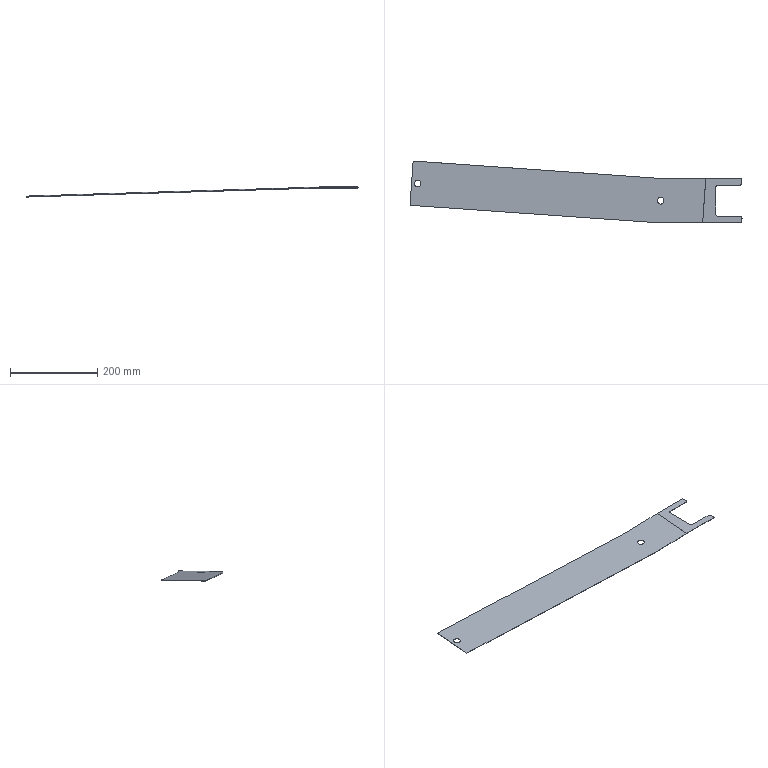Part | SolidWorks | features BaseBody 1 | 1 solid | 28 faces | box 762.872 x 142.38 x 23.327 mm | volume 58351 mm3 | plane 16 | cylinder 10 | spline 2 | commonest cylinder face diameters 10 x4 15.3 x4 2 x1 3.6 x1
STEP:
#1=CARTESIAN_POINT('',(1.188,13.037,-3.513));
#2=VERTEX_POINT('',#1);
#3=CARTESIAN_POINT('',(-14.105,13.037,-3.999));
#4=VERTEX_POINT('',#3);
#5=CARTESIAN_POINT('',(-6.458,13.037,-3.756));
#6=DIRECTION('',(0.03175,0.01522,-0.9994));
#7=DIRECTION('',(0.9995,0.,0.03176));
#8=AXIS2_PLACEMENT_3D('',#5,#6,#7);
#9=CIRCLE('',#8,7.65);
#10=EDGE_CURVE('',#2,#4,#9,.T.);
#11=ORIENTED_EDGE('',*,*,#10,.T.);
#12=CARTESIAN_POINT('',(-14.13,13.025,-3.199));
#13=VERTEX_POINT('',#12);
#14=CARTESIAN_POINT('',(-14.105,13.037,-3.999));
#15=DIRECTION('',(-0.03175,-0.01522,0.9994));
#16=VECTOR('',#15,1000.);
#17=LINE('',#14,#16);
#18=EDGE_CURVE('',#4,#13,#17,.T.);
#19=ORIENTED_EDGE('',*,*,#18,.T.);
#20=CARTESIAN_POINT('',(1.162,13.025,-2.713));
#21=VERTEX_POINT('',#20);
#22=CARTESIAN_POINT('',(-6.484,13.025,-2.956));
#23=DIRECTION('',(-0.03175,-0.01522,0.9994));
#24=DIRECTION('',(0.9995,0.,0.03176));
#25=AXIS2_PLACEMENT_3D('',#22,#23,#24);
#26=CIRCLE('',#25,7.65);
#27=EDGE_CURVE('',#13,#21,#26,.T.);
#28=ORIENTED_EDGE('',*,*,#27,.T.);
#29=CARTESIAN_POINT('',(1.188,13.037,-3.513));
#30=DIRECTION('',(-0.03175,-0.01522,0.9994));
#31=VECTOR('',#30,1000.);
#32=LINE('',#29,#31);
#33=EDGE_CURVE('',#2,#21,#32,.T.);
#34=ORIENTED_EDGE('',*,*,#33,.F.);
#35=EDGE_LOOP('',(#11,#19,#28,#34));
#36=FACE_OUTER_BOUND('',#35,.T.);
#37=CARTESIAN_POINT('',(-6.458,13.037,-3.756));
#38=DIRECTION('',(-0.03175,-0.01522,0.9994));
#39=DIRECTION('',(0.9995,0.,0.03176));
#40=AXIS2_PLACEMENT_3D('',#37,#38,#39);
#41=CYLINDRICAL_SURFACE('',#40,7.65);
#42=ADVANCED_FACE('',(#36),#41,.F.);
#43=CARTESIAN_POINT('',(-557.165,52.386,-20.653));
#44=VERTEX_POINT('',#43);
#45=CARTESIAN_POINT('',(-572.457,52.386,-21.139));
#46=VERTEX_POINT('',#45);
#47=CARTESIAN_POINT('',(-564.811,52.386,-20.896));
#48=DIRECTION('',(0.03175,0.01522,-0.9994));
#49=DIRECTION('',(0.9995,0.,0.03176));
#50=AXIS2_PLACEMENT_3D('',#47,#48,#49);
#51=CIRCLE('',#50,7.65);
#52=EDGE_CURVE('',#44,#46,#51,.T.);
#53=ORIENTED_EDGE('',*,*,#52,.T.);
#54=CARTESIAN_POINT('',(-572.483,52.374,-20.34));
#55=VERTEX_POINT('',#54);
#56=CARTESIAN_POINT('',(-572.457,52.386,-21.139));
#57=DIRECTION('',(-0.03175,-0.01522,0.9994));
#58=VECTOR('',#57,1000.);
#59=LINE('',#56,#58);
#60=EDGE_CURVE('',#46,#55,#59,.T.);
#61=ORIENTED_EDGE('',*,*,#60,.T.);
#62=CARTESIAN_POINT('',(-557.191,52.374,-19.854));
#63=VERTEX_POINT('',#62);
#64=CARTESIAN_POINT('',(-564.837,52.374,-20.097));
#65=DIRECTION('',(0.03175,0.01522,-0.9994));
#66=DIRECTION('',(0.9995,0.,0.03176));
#67=AXIS2_PLACEMENT_3D('',#64,#65,#66);
#68=CIRCLE('',#67,7.65);
#69=EDGE_CURVE('',#63,#55,#68,.T.);
#70=ORIENTED_EDGE('',*,*,#69,.F.);
#71=CARTESIAN_POINT('',(-557.165,52.386,-20.653));
#72=DIRECTION('',(-0.03175,-0.01522,0.9994));
#73=VECTOR('',#72,1000.);
#74=LINE('',#71,#73);
#75=EDGE_CURVE('',#44,#63,#74,.T.);
#76=ORIENTED_EDGE('',*,*,#75,.F.);
#77=EDGE_LOOP('',(#53,#61,#70,#76));
#78=FACE_OUTER_BOUND('',#77,.T.);
#79=CARTESIAN_POINT('',(-564.811,52.386,-20.896));
#80=DIRECTION('',(-0.03175,-0.01522,0.9994));
#81=DIRECTION('',(0.9995,0.,0.03176));
#82=AXIS2_PLACEMENT_3D('',#79,#80,#81);
#83=CYLINDRICAL_SURFACE('',#82,7.65);
#84=ADVANCED_FACE('',(#78),#83,.F.);
#85=ORIENTED_EDGE('',*,*,#18,.F.);
#86=CARTESIAN_POINT('',(-6.458,13.037,-3.756));
#87=DIRECTION('',(0.03175,0.01522,-0.9994));
#88=DIRECTION('',(0.9995,0.,0.03176));
#89=AXIS2_PLACEMENT_3D('',#86,#87,#88);
#90=CIRCLE('',#89,7.65);
#91=EDGE_CURVE('',#4,#2,#90,.T.);
#92=ORIENTED_EDGE('',*,*,#91,.T.);
#93=ORIENTED_EDGE('',*,*,#33,.T.);
#94=CARTESIAN_POINT('',(-6.484,13.025,-2.956));
#95=DIRECTION('',(-0.03175,-0.01522,0.9994));
#96=DIRECTION('',(0.9995,0.,0.03176));
#97=AXIS2_PLACEMENT_3D('',#94,#95,#96);
#98=CIRCLE('',#97,7.65);
#99=EDGE_CURVE('',#21,#13,#98,.T.);
#100=ORIENTED_EDGE('',*,*,#99,.T.);
#101=EDGE_LOOP('',(#85,#92,#93,#100));
#102=FACE_OUTER_BOUND('',#101,.T.);
#103=CARTESIAN_POINT('',(-6.458,13.037,-3.756));
#104=DIRECTION('',(-0.03175,-0.01522,0.9994));
#105=DIRECTION('',(0.9995,0.,0.03176));
#106=AXIS2_PLACEMENT_3D('',#103,#104,#105);
#107=CYLINDRICAL_SURFACE('',#106,7.65);
#108=ADVANCED_FACE('',(#102),#107,.F.);
#109=ORIENTED_EDGE('',*,*,#69,.T.);
#110=CARTESIAN_POINT('',(-564.837,52.374,-20.097));
#111=DIRECTION('',(0.03175,0.01522,-0.9994));
#112=DIRECTION('',(0.9995,0.,0.03176));
#113=AXIS2_PLACEMENT_3D('',#110,#111,#112);
#114=CIRCLE('',#113,7.65);
#115=EDGE_CURVE('',#55,#63,#114,.T.);
#116=ORIENTED_EDGE('',*,*,#115,.T.);
#117=EDGE_LOOP('',(#109,#116));
#118=FACE_BOUND('',#117,.T.);
#119=ORIENTED_EDGE('',*,*,#99,.F.);
#120=ORIENTED_EDGE('',*,*,#27,.F.);
#121=EDGE_LOOP('',(#119,#120));
#122=FACE_BOUND('',#121,.T.);
#123=CARTESIAN_POINT('',(-582.353,2.49,-21.413));
#124=VERTEX_POINT('',#123);
#125=CARTESIAN_POINT('',(-6.526,-38.091,-3.736));
#126=VERTEX_POINT('',#125);
#127=CARTESIAN_POINT('',(-582.353,2.49,-21.413));
#128=DIRECTION('',(0.9971,-0.07027,0.03061));
#129=VECTOR('',#128,1000.);
#130=LINE('',#127,#129);
#131=EDGE_CURVE('',#124,#126,#130,.T.);
#132=ORIENTED_EDGE('',*,*,#131,.T.);
#133=CARTESIAN_POINT('',(90.113,-38.141,-0.6667));
#134=VERTEX_POINT('',#133);
#135=CARTESIAN_POINT('',(-242.556,-37.968,-11.233));
#136=DIRECTION('',(0.9995,-0.0005189,0.03175));
#137=VECTOR('',#136,1000.);
#138=LINE('',#135,#137);
#139=EDGE_CURVE('',#126,#134,#138,.T.);
#140=ORIENTED_EDGE('',*,*,#139,.T.);
#141=CARTESIAN_POINT('',(97.245,63.844,1.113));
#142=VERTEX_POINT('',#141);
#143=CARTESIAN_POINT('',(90.113,-38.141,-0.6667));
#144=DIRECTION('',(0.06976,0.9974,0.01741));
#145=VECTOR('',#144,1000.);
#146=LINE('',#143,#145);
#147=EDGE_CURVE('',#134,#142,#146,.T.);
#148=ORIENTED_EDGE('',*,*,#147,.T.);
#149=CARTESIAN_POINT('',(-2.962,63.896,-2.069));
#150=VERTEX_POINT('',#149);
#151=CARTESIAN_POINT('',(-242.553,64.02,-9.68));
#152=DIRECTION('',(-0.9995,0.0005189,-0.03175));
#153=VECTOR('',#152,1000.);
#154=LINE('',#151,#153);
#155=EDGE_CURVE('',#142,#150,#154,.T.);
#156=ORIENTED_EDGE('',*,*,#155,.T.);
#157=CARTESIAN_POINT('',(-575.238,104.226,-19.637));
#158=VERTEX_POINT('',#157);
#159=CARTESIAN_POINT('',(-2.962,63.896,-2.069));
#160=DIRECTION('',(-0.9971,0.07027,-0.03061));
#161=VECTOR('',#160,1000.);
#162=LINE('',#159,#161);
#163=EDGE_CURVE('',#150,#158,#162,.T.);
#164=ORIENTED_EDGE('',*,*,#163,.T.);
#165=CARTESIAN_POINT('',(-575.238,104.226,-19.637));
#166=DIRECTION('',(-0.06976,-0.9974,-0.01741));
#167=VECTOR('',#166,1000.);
#168=LINE('',#165,#167);
#169=EDGE_CURVE('',#158,#124,#168,.T.);
#170=ORIENTED_EDGE('',*,*,#169,.T.);
#171=EDGE_LOOP('',(#132,#140,#148,#156,#164,#170));
#172=FACE_OUTER_BOUND('',#171,.T.);
#173=CARTESIAN_POINT('',(-586.427,105.084,-19.98));
#174=DIRECTION('',(-0.03175,-0.01522,0.9994));
#175=DIRECTION('',(-0.00003526,-0.9999,-0.01523));
#176=AXIS2_PLACEMENT_3D('',#173,#174,#175);
#177=PLANE('',#176);
#178=ADVANCED_FACE('',(#118,#122,#172),#177,.T.);
#179=ORIENTED_EDGE('',*,*,#52,.F.);
#180=CARTESIAN_POINT('',(-564.811,52.386,-20.896));
#181=DIRECTION('',(0.03175,0.01522,-0.9994));
#182=DIRECTION('',(0.9995,0.,0.03176));
#183=AXIS2_PLACEMENT_3D('',#180,#181,#182);
#184=CIRCLE('',#183,7.65);
#185=EDGE_CURVE('',#46,#44,#184,.T.);
#186=ORIENTED_EDGE('',*,*,#185,.F.);
#187=EDGE_LOOP('',(#179,#186));
#188=FACE_BOUND('',#187,.T.);
#189=ORIENTED_EDGE('',*,*,#10,.F.);
#190=ORIENTED_EDGE('',*,*,#91,.F.);
#191=EDGE_LOOP('',(#189,#190));
#192=FACE_BOUND('',#191,.T.);
#193=CARTESIAN_POINT('',(90.138,-38.129,-1.466));
#194=VERTEX_POINT('',#193);
#195=CARTESIAN_POINT('',(97.271,63.856,0.314));
#196=VERTEX_POINT('',#195);
#197=CARTESIAN_POINT('',(90.095,-38.741,-1.477));
#198=DIRECTION('',(0.06976,0.9974,0.01741));
#199=VECTOR('',#198,1000.);
#200=LINE('',#197,#199);
#201=EDGE_CURVE('',#194,#196,#200,.T.);
#202=ORIENTED_EDGE('',*,*,#201,.F.);
#203=CARTESIAN_POINT('',(-6.5,-38.079,-4.536));
#204=VERTEX_POINT('',#203);
#205=CARTESIAN_POINT('',(-242.531,-37.956,-12.033));
#206=DIRECTION('',(0.9995,-0.0005189,0.03175));
#207=VECTOR('',#206,1000.);
#208=LINE('',#205,#207);
#209=EDGE_CURVE('',#204,#194,#208,.T.);
#210=ORIENTED_EDGE('',*,*,#209,.F.);
#211=CARTESIAN_POINT('',(-582.328,2.502,-22.213));
#212=VERTEX_POINT('',#211);
#213=CARTESIAN_POINT('',(-582.328,2.502,-22.213));
#214=DIRECTION('',(0.9971,-0.07027,0.03061));
#215=VECTOR('',#214,1000.);
#216=LINE('',#213,#215);
#217=EDGE_CURVE('',#212,#204,#216,.T.);
#218=ORIENTED_EDGE('',*,*,#217,.F.);
#219=CARTESIAN_POINT('',(-575.213,104.238,-20.437));
#220=VERTEX_POINT('',#219);
#221=CARTESIAN_POINT('',(-575.213,104.238,-20.437));
#222=DIRECTION('',(-0.06976,-0.9974,-0.01741));
#223=VECTOR('',#222,1000.);
#224=LINE('',#221,#223);
#225=EDGE_CURVE('',#220,#212,#224,.T.);
#226=ORIENTED_EDGE('',*,*,#225,.F.);
#227=CARTESIAN_POINT('',(-2.937,63.908,-2.869));
#228=VERTEX_POINT('',#227);
#229=CARTESIAN_POINT('',(-2.937,63.908,-2.869));
#230=DIRECTION('',(-0.9971,0.07027,-0.03061));
#231=VECTOR('',#230,1000.);
#232=LINE('',#229,#231);
#233=EDGE_CURVE('',#228,#220,#232,.T.);
#234=ORIENTED_EDGE('',*,*,#233,.F.);
#235=CARTESIAN_POINT('',(-242.527,64.032,-10.479));
#236=DIRECTION('',(-0.9995,0.0005189,-0.03175));
#237=VECTOR('',#236,1000.);
#238=LINE('',#235,#237);
#239=EDGE_CURVE('',#196,#228,#238,.T.);
#240=ORIENTED_EDGE('',*,*,#239,.F.);
#241=EDGE_LOOP('',(#202,#210,#218,#226,#234,#240));
#242=FACE_OUTER_BOUND('',#241,.T.);
#243=CARTESIAN_POINT('',(-586.402,105.096,-20.779));
#244=DIRECTION('',(-0.03175,-0.01522,0.9994));
#245=DIRECTION('',(-0.00003526,-0.9999,-0.01523));
#246=AXIS2_PLACEMENT_3D('',#243,#244,#245);
#247=PLANE('',#246);
#248=ADVANCED_FACE('',(#188,#192,#242),#247,.F.);
#249=ORIENTED_EDGE('',*,*,#60,.F.);
#250=ORIENTED_EDGE('',*,*,#185,.T.);
#251=ORIENTED_EDGE('',*,*,#75,.T.);
#252=ORIENTED_EDGE('',*,*,#115,.F.);
#253=EDGE_LOOP('',(#249,#250,#251,#252));
#254=FACE_OUTER_BOUND('',#253,.T.);
#255=CARTESIAN_POINT('',(-564.811,52.386,-20.896));
#256=DIRECTION('',(-0.03175,-0.01522,0.9994));
#257=DIRECTION('',(0.9995,0.,0.03176));
#258=AXIS2_PLACEMENT_3D('',#255,#256,#257);
#259=CYLINDRICAL_SURFACE('',#258,7.65);
#260=ADVANCED_FACE('',(#254),#259,.F.);
#261=CARTESIAN_POINT('',(90.125,-38.135,-1.066));
#262=DIRECTION('',(0.03175,0.01522,-0.9994));
#263=VECTOR('',#262,1000.);
#264=LINE('',#261,#263);
#265=EDGE_CURVE('',#134,#194,#264,.T.);
#266=ORIENTED_EDGE('',*,*,#265,.F.);
#267=ORIENTED_EDGE('',*,*,#139,.F.);
#268=CARTESIAN_POINT('',(-6.513,-38.085,-4.136));
#269=DIRECTION('',(-0.03175,-0.01522,0.9994));
#270=VECTOR('',#269,1000.);
#271=LINE('',#268,#270);
#272=EDGE_CURVE('',#204,#126,#271,.T.);
#273=ORIENTED_EDGE('',*,*,#272,.F.);
#274=ORIENTED_EDGE('',*,*,#209,.T.);
#275=EDGE_LOOP('',(#266,#267,#273,#274));
#276=FACE_OUTER_BOUND('',#275,.T.);
#277=CARTESIAN_POINT('',(-6.5,-38.079,-4.536));
#278=DIRECTION('',(0.00003526,0.9999,0.01523));
#279=DIRECTION('',(-0.03175,-0.01522,0.9994));
#280=AXIS2_PLACEMENT_3D('',#277,#278,#279);
#281=PLANE('',#280);
#282=ADVANCED_FACE('',(#276),#281,.F.);
#283=CARTESIAN_POINT('',(-582.328,2.502,-22.213));
#284=DIRECTION('',(-0.03175,-0.01522,0.9994));
#285=VECTOR('',#284,1000.);
#286=LINE('',#283,#285);
#287=EDGE_CURVE('',#212,#124,#286,.T.);
#288=ORIENTED_EDGE('',*,*,#287,.F.);
#289=ORIENTED_EDGE('',*,*,#217,.T.);
#290=ORIENTED_EDGE('',*,*,#272,.T.);
#291=ORIENTED_EDGE('',*,*,#131,.F.);
#292=EDGE_LOOP('',(#288,#289,#290,#291));
#293=FACE_OUTER_BOUND('',#292,.T.);
#294=CARTESIAN_POINT('',(-3.044,-38.322,-4.434));
#295=DIRECTION('',(0.06976,0.9974,0.01741));
#296=DIRECTION('',(-0.997,0.07028,-0.03182));
#297=AXIS2_PLACEMENT_3D('',#294,#295,#296);
#298=PLANE('',#297);
#299=ADVANCED_FACE('',(#293),#298,.F.);
#300=CARTESIAN_POINT('',(-575.213,104.238,-20.437));
#301=DIRECTION('',(-0.03175,-0.01522,0.9994));
#302=VECTOR('',#301,1000.);
#303=LINE('',#300,#302);
#304=EDGE_CURVE('',#220,#158,#303,.T.);
#305=ORIENTED_EDGE('',*,*,#304,.F.);
#306=ORIENTED_EDGE('',*,*,#225,.T.);
#307=ORIENTED_EDGE('',*,*,#287,.T.);
#308=ORIENTED_EDGE('',*,*,#169,.F.);
#309=EDGE_LOOP('',(#305,#306,#307,#308));
#310=FACE_OUTER_BOUND('',#309,.T.);
#311=CARTESIAN_POINT('',(-582.371,1.878,-22.228));
#312=DIRECTION('',(0.9971,-0.07027,0.03061));
#313=DIRECTION('',(0.0703,0.9975,0.000008145));
#314=AXIS2_PLACEMENT_3D('',#311,#312,#313);
#315=PLANE('',#314);
#316=ADVANCED_FACE('',(#310),#315,.F.);
#317=CARTESIAN_POINT('',(-2.962,63.896,-2.069));
#318=DIRECTION('',(-0.03175,-0.01522,0.9994));
#319=VECTOR('',#318,1000.);
#320=LINE('',#317,#319);
#321=EDGE_CURVE('',#228,#150,#320,.T.);
#322=ORIENTED_EDGE('',*,*,#321,.F.);
#323=ORIENTED_EDGE('',*,*,#233,.T.);
#324=ORIENTED_EDGE('',*,*,#304,.T.);
#325=ORIENTED_EDGE('',*,*,#163,.F.);
#326=EDGE_LOOP('',(#322,#323,#324,#325));
#327=FACE_OUTER_BOUND('',#326,.T.);
#328=CARTESIAN_POINT('',(-578.623,104.491,-21.254));
#329=DIRECTION('',(-0.06976,-0.9974,-0.01741));
#330=DIRECTION('',(0.997,-0.07028,0.03182));
#331=AXIS2_PLACEMENT_3D('',#328,#329,#330);
#332=PLANE('',#331);
#333=ADVANCED_FACE('',(#327),#332,.F.);
#334=CARTESIAN_POINT('',(97.258,63.85,0.7137));
#335=DIRECTION('',(-0.03175,-0.01522,0.9994));
#336=VECTOR('',#335,1000.);
#337=LINE('',#334,#336);
#338=EDGE_CURVE('',#196,#142,#337,.T.);
#339=ORIENTED_EDGE('',*,*,#338,.F.);
#340=ORIENTED_EDGE('',*,*,#239,.T.);
#341=ORIENTED_EDGE('',*,*,#321,.T.);
#342=ORIENTED_EDGE('',*,*,#155,.F.);
#343=EDGE_LOOP('',(#339,#340,#341,#342));
#344=FACE_OUTER_BOUND('',#343,.T.);
#345=CARTESIAN_POINT('',(-2.962,63.896,-2.069));
#346=DIRECTION('',(-0.00003526,-0.9999,-0.01523));
#347=DIRECTION('',(0.03175,0.01522,-0.9994));
#348=AXIS2_PLACEMENT_3D('',#345,#346,#347);
#349=PLANE('',#348);
#350=ADVANCED_FACE('',(#344),#349,.F.);
#351=CARTESIAN_POINT('',(97.303,63.843,1.114));
#352=VERTEX_POINT('',#351);
#353=CARTESIAN_POINT('',(90.17,-38.142,-0.6658));
#354=VERTEX_POINT('',#353);
#355=CARTESIAN_POINT('',(93.736,12.849,0.2243));
#356=DIRECTION('',(-0.06976,-0.9974,-0.01741));
#357=VECTOR('',#356,1000.);
#358=LINE('',#355,#357);
#359=EDGE_CURVE('',#352,#354,#358,.T.);
#360=ORIENTED_EDGE('',*,*,#359,.F.);
#361=CARTESIAN_POINT('',(97.245,63.844,1.113));
#362=CARTESIAN_POINT('',(97.264,63.843,1.114));
#363=CARTESIAN_POINT('',(97.283,63.843,1.114));
#364=CARTESIAN_POINT('',(97.303,63.843,1.114));
#365=B_SPLINE_CURVE_WITH_KNOTS('',3,(#361,#362,#363,#364),.UNSPECIFIED.,.F.,.F.,(4,4),(0.,1.),.UNSPECIFIED.);
#366=EDGE_CURVE('',#142,#352,#365,.T.);
#367=ORIENTED_EDGE('',*,*,#366,.F.);
#368=ORIENTED_EDGE('',*,*,#147,.F.);
#369=CARTESIAN_POINT('',(90.17,-38.142,-0.6658));
#370=CARTESIAN_POINT('',(90.151,-38.141,-0.6658));
#371=CARTESIAN_POINT('',(90.132,-38.141,-0.6661));
#372=CARTESIAN_POINT('',(90.113,-38.141,-0.6667));
#373=B_SPLINE_CURVE_WITH_KNOTS('',3,(#369,#370,#371,#372),.UNSPECIFIED.,.F.,.F.,(4,4),(0.,1.),.UNSPECIFIED.);
#374=EDGE_CURVE('',#354,#134,#373,.T.);
#375=ORIENTED_EDGE('',*,*,#374,.F.);
#376=EDGE_LOOP('',(#360,#367,#368,#375));
#377=FACE_OUTER_BOUND('',#376,.T.);
#378=CARTESIAN_POINT('',(90.127,-38.725,-2.476));
#379=DIRECTION('',(0.06976,0.9974,0.01741));
#380=DIRECTION('',(-0.9976,0.06977,0.));
#381=AXIS2_PLACEMENT_3D('',#378,#379,#380);
#382=CYLINDRICAL_SURFACE('',#381,1.8);
#383=ADVANCED_FACE('',(#377),#382,.T.);
#384=CARTESIAN_POINT('',(97.303,63.857,0.3145));
#385=VERTEX_POINT('',#384);
#386=CARTESIAN_POINT('',(97.271,63.856,0.314));
#387=CARTESIAN_POINT('',(97.281,63.856,0.3143));
#388=CARTESIAN_POINT('',(97.292,63.856,0.3145));
#389=CARTESIAN_POINT('',(97.303,63.857,0.3145));
#390=B_SPLINE_CURVE_WITH_KNOTS('',3,(#386,#387,#388,#389),.UNSPECIFIED.,.F.,.F.,(4,4),(0.000004021,1.),.UNSPECIFIED.);
#391=EDGE_CURVE('',#196,#385,#390,.T.);
#392=ORIENTED_EDGE('',*,*,#391,.T.);
#393=CARTESIAN_POINT('',(90.17,-38.128,-1.466));
#394=VERTEX_POINT('',#393);
#395=CARTESIAN_POINT('',(93.736,12.863,-0.5756));
#396=DIRECTION('',(-0.06976,-0.9974,-0.01741));
#397=VECTOR('',#396,1000.);
#398=LINE('',#395,#397);
#399=EDGE_CURVE('',#385,#394,#398,.T.);
#400=ORIENTED_EDGE('',*,*,#399,.T.);
#401=CARTESIAN_POINT('',(90.17,-38.128,-1.466));
#402=CARTESIAN_POINT('',(90.159,-38.128,-1.466));
#403=CARTESIAN_POINT('',(90.149,-38.128,-1.466));
#404=CARTESIAN_POINT('',(90.138,-38.129,-1.466));
#405=B_SPLINE_CURVE_WITH_KNOTS('',3,(#401,#402,#403,#404),.UNSPECIFIED.,.F.,.F.,(4,4),(0.,1.),.UNSPECIFIED.);
#406=EDGE_CURVE('',#394,#194,#405,.T.);
#407=ORIENTED_EDGE('',*,*,#406,.T.);
#408=ORIENTED_EDGE('',*,*,#201,.T.);
#409=EDGE_LOOP('',(#392,#400,#407,#408));
#410=FACE_OUTER_BOUND('',#409,.T.);
#411=CARTESIAN_POINT('',(90.127,-38.725,-2.476));
#412=DIRECTION('',(0.06976,0.9974,0.01741));
#413=DIRECTION('',(-0.9976,0.06977,0.));
#414=AXIS2_PLACEMENT_3D('',#411,#412,#413);
#415=CYLINDRICAL_SURFACE('',#414,1.);
#416=ADVANCED_FACE('',(#410),#415,.F.);
#417=ORIENTED_EDGE('',*,*,#374,.T.);
#418=ORIENTED_EDGE('',*,*,#265,.T.);
#419=ORIENTED_EDGE('',*,*,#406,.F.);
#420=CARTESIAN_POINT('',(90.17,-38.135,-1.066));
#421=DIRECTION('',(0.,-0.01745,0.9998));
#422=VECTOR('',#421,1000.);
#423=LINE('',#420,#422);
#424=EDGE_CURVE('',#394,#354,#423,.T.);
#425=ORIENTED_EDGE('',*,*,#424,.T.);
#426=EDGE_LOOP('',(#417,#418,#419,#425));
#427=FACE_OUTER_BOUND('',#426,.T.);
#428=CARTESIAN_POINT('',(90.17,-38.142,-0.6658));
#429=CARTESIAN_POINT('',(90.151,-38.141,-0.6658));
#430=CARTESIAN_POINT('',(90.132,-38.141,-0.6661));
#431=CARTESIAN_POINT('',(90.113,-38.141,-0.6667));
#432=CARTESIAN_POINT('',(90.17,-38.128,-1.466));
#433=CARTESIAN_POINT('',(90.159,-38.128,-1.466));
#434=CARTESIAN_POINT('',(90.149,-38.128,-1.466));
#435=CARTESIAN_POINT('',(90.138,-38.129,-1.466));
#436=B_SPLINE_SURFACE_WITH_KNOTS('',1,3,((#428,#429,#430,#431),(#432,#433,#434,#435)),.UNSPECIFIED.,.F.,.F.,.F.,(2,2),(4,4),(0.,1.),(0.,1.),.UNSPECIFIED.);
#437=ADVANCED_FACE('',(#427),#436,.F.);
#438=ORIENTED_EDGE('',*,*,#366,.T.);
#439=CARTESIAN_POINT('',(97.303,63.85,0.7144));
#440=DIRECTION('',(0.,0.01745,-0.9998));
#441=VECTOR('',#440,1000.);
#442=LINE('',#439,#441);
#443=EDGE_CURVE('',#352,#385,#442,.T.);
#444=ORIENTED_EDGE('',*,*,#443,.T.);
#445=ORIENTED_EDGE('',*,*,#391,.F.);
#446=ORIENTED_EDGE('',*,*,#338,.T.);
#447=EDGE_LOOP('',(#438,#444,#445,#446));
#448=FACE_OUTER_BOUND('',#447,.T.);
#449=CARTESIAN_POINT('',(97.245,63.844,1.113));
#450=CARTESIAN_POINT('',(97.264,63.843,1.114));
#451=CARTESIAN_POINT('',(97.283,63.843,1.114));
#452=CARTESIAN_POINT('',(97.303,63.843,1.114));
#453=CARTESIAN_POINT('',(97.271,63.856,0.314));
#454=CARTESIAN_POINT('',(97.281,63.856,0.3143));
#455=CARTESIAN_POINT('',(97.292,63.856,0.3145));
#456=CARTESIAN_POINT('',(97.303,63.857,0.3145));
#457=B_SPLINE_SURFACE_WITH_KNOTS('',1,3,((#449,#450,#451,#452),(#453,#454,#455,#456)),.UNSPECIFIED.,.F.,.F.,.F.,(2,2),(4,4),(0.,1.),(0.,1.),.UNSPECIFIED.);
#458=ADVANCED_FACE('',(#448),#457,.F.);
#459=CARTESIAN_POINT('',(175.519,48.845,0.8526));
#460=VERTEX_POINT('',#459);
#461=CARTESIAN_POINT('',(180.519,53.844,0.9399));
#462=VERTEX_POINT('',#461);
#463=CARTESIAN_POINT('',(175.519,53.844,0.9399));
#464=DIRECTION('',(0.,-0.01745,0.9998));
#465=DIRECTION('',(0.,-0.9998,-0.01745));
#466=AXIS2_PLACEMENT_3D('',#463,#464,#465);
#467=CIRCLE('',#466,5.);
#468=EDGE_CURVE('',#460,#462,#467,.T.);
#469=ORIENTED_EDGE('',*,*,#468,.T.);
#470=CARTESIAN_POINT('',(180.519,63.843,1.114));
#471=VERTEX_POINT('',#470);
#472=CARTESIAN_POINT('',(180.519,12.85,0.2243));
#473=DIRECTION('',(0.,0.9998,0.01745));
#474=VECTOR('',#473,1000.);
#475=LINE('',#472,#474);
#476=EDGE_CURVE('',#462,#471,#475,.T.);
#477=ORIENTED_EDGE('',*,*,#476,.T.);
#478=CARTESIAN_POINT('',(135.073,63.843,1.114));
#479=DIRECTION('',(-1.,0.,0.));
#480=VECTOR('',#479,1000.);
#481=LINE('',#478,#480);
#482=EDGE_CURVE('',#471,#352,#481,.T.);
#483=ORIENTED_EDGE('',*,*,#482,.T.);
#484=ORIENTED_EDGE('',*,*,#359,.T.);
#485=CARTESIAN_POINT('',(180.519,-38.142,-0.6658));
#486=VERTEX_POINT('',#485);
#487=CARTESIAN_POINT('',(135.073,-38.142,-0.6658));
#488=DIRECTION('',(1.,0.,0.));
#489=VECTOR('',#488,1000.);
#490=LINE('',#487,#489);
#491=EDGE_CURVE('',#354,#486,#490,.T.);
#492=ORIENTED_EDGE('',*,*,#491,.T.);
#493=CARTESIAN_POINT('',(180.519,-28.143,-0.4912));
#494=VERTEX_POINT('',#493);
#495=CARTESIAN_POINT('',(180.519,12.85,0.2243));
#496=DIRECTION('',(0.,0.9998,0.01745));
#497=VECTOR('',#496,1000.);
#498=LINE('',#495,#497);
#499=EDGE_CURVE('',#486,#494,#498,.T.);
#500=ORIENTED_EDGE('',*,*,#499,.T.);
#501=CARTESIAN_POINT('',(175.519,-23.144,-0.404));
#502=VERTEX_POINT('',#501);
#503=CARTESIAN_POINT('',(175.519,-28.143,-0.4912));
#504=DIRECTION('',(0.,-0.01745,0.9998));
#505=DIRECTION('',(0.,-0.9998,-0.01745));
#506=AXIS2_PLACEMENT_3D('',#503,#504,#505);
#507=CIRCLE('',#506,5.);
#508=EDGE_CURVE('',#494,#502,#507,.T.);
#509=ORIENTED_EDGE('',*,*,#508,.T.);
#510=CARTESIAN_POINT('',(125.519,-23.144,-0.404));
#511=VERTEX_POINT('',#510);
#512=CARTESIAN_POINT('',(135.073,-23.144,-0.404));
#513=DIRECTION('',(-1.,0.,0.));
#514=VECTOR('',#513,1000.);
#515=LINE('',#512,#514);
#516=EDGE_CURVE('',#502,#511,#515,.T.);
#517=ORIENTED_EDGE('',*,*,#516,.T.);
#518=CARTESIAN_POINT('',(120.519,-18.145,-0.3167));
#519=VERTEX_POINT('',#518);
#520=CARTESIAN_POINT('',(125.519,-18.145,-0.3167));
#521=DIRECTION('',(0.,0.01745,-0.9998));
#522=DIRECTION('',(0.,-0.9998,-0.01745));
#523=AXIS2_PLACEMENT_3D('',#520,#521,#522);
#524=CIRCLE('',#523,5.);
#525=EDGE_CURVE('',#511,#519,#524,.T.);
#526=ORIENTED_EDGE('',*,*,#525,.T.);
#527=CARTESIAN_POINT('',(120.519,43.846,0.7653));
#528=VERTEX_POINT('',#527);
#529=CARTESIAN_POINT('',(120.519,12.85,0.2243));
#530=DIRECTION('',(0.,0.9998,0.01745));
#531=VECTOR('',#530,1000.);
#532=LINE('',#529,#531);
#533=EDGE_CURVE('',#519,#528,#532,.T.);
#534=ORIENTED_EDGE('',*,*,#533,.T.);
#535=CARTESIAN_POINT('',(125.519,48.845,0.8526));
#536=VERTEX_POINT('',#535);
#537=CARTESIAN_POINT('',(125.519,43.846,0.7653));
#538=DIRECTION('',(0.,0.01745,-0.9998));
#539=DIRECTION('',(0.,-0.9998,-0.01745));
#540=AXIS2_PLACEMENT_3D('',#537,#538,#539);
#541=CIRCLE('',#540,5.);
#542=EDGE_CURVE('',#528,#536,#541,.T.);
#543=ORIENTED_EDGE('',*,*,#542,.T.);
#544=CARTESIAN_POINT('',(135.073,48.845,0.8526));
#545=DIRECTION('',(1.,0.,0.));
#546=VECTOR('',#545,1000.);
#547=LINE('',#544,#546);
#548=EDGE_CURVE('',#536,#460,#547,.T.);
#549=ORIENTED_EDGE('',*,*,#548,.T.);
#550=EDGE_LOOP('',(#469,#477,#483,#484,#492,#500,#509,#517,#526,#534,#543,#549));
#551=FACE_OUTER_BOUND('',#550,.T.);
#552=CARTESIAN_POINT('',(89.628,63.843,1.114));
#553=DIRECTION('',(0.,-0.01745,0.9998));
#554=DIRECTION('',(0.,-0.9998,-0.01745));
#555=AXIS2_PLACEMENT_3D('',#552,#553,#554);
#556=PLANE('',#555);
#557=ADVANCED_FACE('',(#551),#556,.T.);
#558=CARTESIAN_POINT('',(180.519,63.857,0.3145));
#559=VERTEX_POINT('',#558);
#560=CARTESIAN_POINT('',(135.073,63.857,0.3145));
#561=DIRECTION('',(-1.,0.,0.));
#562=VECTOR('',#561,1000.);
#563=LINE('',#560,#562);
#564=EDGE_CURVE('',#559,#385,#563,.T.);
#565=ORIENTED_EDGE('',*,*,#564,.F.);
#566=CARTESIAN_POINT('',(180.519,53.858,0.14));
#567=VERTEX_POINT('',#566);
#568=CARTESIAN_POINT('',(180.519,12.864,-0.5756));
#569=DIRECTION('',(0.,0.9998,0.01745));
#570=VECTOR('',#569,1000.);
#571=LINE('',#568,#570);
#572=EDGE_CURVE('',#567,#559,#571,.T.);
#573=ORIENTED_EDGE('',*,*,#572,.F.);
#574=CARTESIAN_POINT('',(175.519,48.859,0.05271));
#575=VERTEX_POINT('',#574);
#576=CARTESIAN_POINT('',(175.519,53.858,0.14));
#577=DIRECTION('',(0.,-0.01745,0.9998));
#578=DIRECTION('',(0.,-0.9998,-0.01745));
#579=AXIS2_PLACEMENT_3D('',#576,#577,#578);
#580=CIRCLE('',#579,5.);
#581=EDGE_CURVE('',#575,#567,#580,.T.);
#582=ORIENTED_EDGE('',*,*,#581,.F.);
#583=CARTESIAN_POINT('',(125.519,48.859,0.05271));
#584=VERTEX_POINT('',#583);
#585=CARTESIAN_POINT('',(135.073,48.859,0.05271));
#586=DIRECTION('',(1.,0.,0.));
#587=VECTOR('',#586,1000.);
#588=LINE('',#585,#587);
#589=EDGE_CURVE('',#584,#575,#588,.T.);
#590=ORIENTED_EDGE('',*,*,#589,.F.);
#591=CARTESIAN_POINT('',(120.519,43.86,-0.03455));
#592=VERTEX_POINT('',#591);
#593=CARTESIAN_POINT('',(125.519,43.86,-0.03455));
#594=DIRECTION('',(0.,0.01745,-0.9998));
#595=DIRECTION('',(0.,-0.9998,-0.01745));
#596=AXIS2_PLACEMENT_3D('',#593,#594,#595);
#597=CIRCLE('',#596,5.);
#598=EDGE_CURVE('',#592,#584,#597,.T.);
#599=ORIENTED_EDGE('',*,*,#598,.F.);
#600=CARTESIAN_POINT('',(120.519,-18.131,-1.117));
#601=VERTEX_POINT('',#600);
#602=CARTESIAN_POINT('',(120.519,12.864,-0.5756));
#603=DIRECTION('',(0.,0.9998,0.01745));
#604=VECTOR('',#603,1000.);
#605=LINE('',#602,#604);
#606=EDGE_CURVE('',#601,#592,#605,.T.);
#607=ORIENTED_EDGE('',*,*,#606,.F.);
#608=CARTESIAN_POINT('',(125.519,-23.13,-1.204));
#609=VERTEX_POINT('',#608);
#610=CARTESIAN_POINT('',(125.519,-18.131,-1.117));
#611=DIRECTION('',(0.,0.01745,-0.9998));
#612=DIRECTION('',(0.,-0.9998,-0.01745));
#613=AXIS2_PLACEMENT_3D('',#610,#611,#612);
#614=CIRCLE('',#613,5.);
#615=EDGE_CURVE('',#609,#601,#614,.T.);
#616=ORIENTED_EDGE('',*,*,#615,.F.);
#617=CARTESIAN_POINT('',(175.519,-23.13,-1.204));
#618=VERTEX_POINT('',#617);
#619=CARTESIAN_POINT('',(135.073,-23.13,-1.204));
#620=DIRECTION('',(-1.,0.,0.));
#621=VECTOR('',#620,1000.);
#622=LINE('',#619,#621);
#623=EDGE_CURVE('',#618,#609,#622,.T.);
#624=ORIENTED_EDGE('',*,*,#623,.F.);
#625=CARTESIAN_POINT('',(180.519,-28.129,-1.291));
#626=VERTEX_POINT('',#625);
#627=CARTESIAN_POINT('',(175.519,-28.129,-1.291));
#628=DIRECTION('',(0.,-0.01745,0.9998));
#629=DIRECTION('',(0.,-0.9998,-0.01745));
#630=AXIS2_PLACEMENT_3D('',#627,#628,#629);
#631=CIRCLE('',#630,5.);
#632=EDGE_CURVE('',#626,#618,#631,.T.);
#633=ORIENTED_EDGE('',*,*,#632,.F.);
#634=CARTESIAN_POINT('',(180.519,-38.128,-1.466));
#635=VERTEX_POINT('',#634);
#636=CARTESIAN_POINT('',(180.519,12.864,-0.5756));
#637=DIRECTION('',(0.,0.9998,0.01745));
#638=VECTOR('',#637,1000.);
#639=LINE('',#636,#638);
#640=EDGE_CURVE('',#635,#626,#639,.T.);
#641=ORIENTED_EDGE('',*,*,#640,.F.);
#642=CARTESIAN_POINT('',(135.073,-38.128,-1.466));
#643=DIRECTION('',(1.,0.,0.));
#644=VECTOR('',#643,1000.);
#645=LINE('',#642,#644);
#646=EDGE_CURVE('',#394,#635,#645,.T.);
#647=ORIENTED_EDGE('',*,*,#646,.F.);
#648=ORIENTED_EDGE('',*,*,#399,.F.);
#649=EDGE_LOOP('',(#565,#573,#582,#590,#599,#607,#616,#624,#633,#641,#647,#648));
#650=FACE_OUTER_BOUND('',#649,.T.);
#651=CARTESIAN_POINT('',(89.628,63.857,0.3145));
#652=DIRECTION('',(0.,-0.01745,0.9998));
#653=DIRECTION('',(0.,-0.9998,-0.01745));
#654=AXIS2_PLACEMENT_3D('',#651,#652,#653);
#655=PLANE('',#654);
#656=ADVANCED_FACE('',(#650),#655,.F.);
#657=CARTESIAN_POINT('',(180.519,53.858,0.14));
#658=DIRECTION('',(0.,-0.01745,0.9998));
#659=VECTOR('',#658,1000.);
#660=LINE('',#657,#659);
#661=EDGE_CURVE('',#567,#462,#660,.T.);
#662=ORIENTED_EDGE('',*,*,#661,.F.);
#663=ORIENTED_EDGE('',*,*,#572,.T.);
#664=CARTESIAN_POINT('',(180.519,63.843,1.114));
#665=DIRECTION('',(0.,0.01745,-0.9998));
#666=VECTOR('',#665,1000.);
#667=LINE('',#664,#666);
#668=EDGE_CURVE('',#471,#559,#667,.T.);
#669=ORIENTED_EDGE('',*,*,#668,.F.);
#670=ORIENTED_EDGE('',*,*,#476,.F.);
#671=EDGE_LOOP('',(#662,#663,#669,#670));
#672=FACE_OUTER_BOUND('',#671,.T.);
#673=CARTESIAN_POINT('',(180.519,53.784,0.1341));
#674=DIRECTION('',(-1.,0.,0.));
#675=DIRECTION('',(0.,0.,1.));
#676=AXIS2_PLACEMENT_3D('',#673,#674,#675);
#677=PLANE('',#676);
#678=ADVANCED_FACE('',(#672),#677,.F.);
#679=CARTESIAN_POINT('',(175.519,48.852,0.4527));
#680=DIRECTION('',(0.,-0.01745,0.9998));
#681=VECTOR('',#680,1000.);
#682=LINE('',#679,#681);
#683=EDGE_CURVE('',#575,#460,#682,.T.);
#684=ORIENTED_EDGE('',*,*,#683,.F.);
#685=ORIENTED_EDGE('',*,*,#581,.T.);
#686=ORIENTED_EDGE('',*,*,#661,.T.);
#687=ORIENTED_EDGE('',*,*,#468,.F.);
#688=EDGE_LOOP('',(#684,#685,#686,#687));
#689=FACE_OUTER_BOUND('',#688,.T.);
#690=CARTESIAN_POINT('',(175.519,53.858,0.14));
#691=DIRECTION('',(0.,-0.01745,0.9998));
#692=DIRECTION('',(0.,-0.9998,-0.01745));
#693=AXIS2_PLACEMENT_3D('',#690,#691,#692);
#694=CYLINDRICAL_SURFACE('',#693,5.);
#695=ADVANCED_FACE('',(#689),#694,.T.);
#696=CARTESIAN_POINT('',(125.519,48.852,0.4527));
#697=DIRECTION('',(0.,-0.01745,0.9998));
#698=VECTOR('',#697,1000.);
#699=LINE('',#696,#698);
#700=EDGE_CURVE('',#584,#536,#699,.T.);
#701=ORIENTED_EDGE('',*,*,#700,.F.);
#702=ORIENTED_EDGE('',*,*,#589,.T.);
#703=ORIENTED_EDGE('',*,*,#683,.T.);
#704=ORIENTED_EDGE('',*,*,#548,.F.);
#705=EDGE_LOOP('',(#701,#702,#703,#704));
#706=FACE_OUTER_BOUND('',#705,.T.);
#707=CARTESIAN_POINT('',(125.519,48.859,0.05271));
#708=DIRECTION('',(0.,0.9998,0.01745));
#709=DIRECTION('',(0.,-0.01745,0.9998));
#710=AXIS2_PLACEMENT_3D('',#707,#708,#709);
#711=PLANE('',#710);
#712=ADVANCED_FACE('',(#706),#711,.F.);
#713=ORIENTED_EDGE('',*,*,#598,.T.);
#714=ORIENTED_EDGE('',*,*,#700,.T.);
#715=ORIENTED_EDGE('',*,*,#542,.F.);
#716=CARTESIAN_POINT('',(120.519,43.853,0.3654));
#717=DIRECTION('',(0.,0.01745,-0.9998));
#718=VECTOR('',#717,1000.);
#719=LINE('',#716,#718);
#720=EDGE_CURVE('',#528,#592,#719,.T.);
#721=ORIENTED_EDGE('',*,*,#720,.T.);
#722=EDGE_LOOP('',(#713,#714,#715,#721));
#723=FACE_OUTER_BOUND('',#722,.T.);
#724=CARTESIAN_POINT('',(125.519,43.86,-0.03455));
#725=DIRECTION('',(0.,-0.01745,0.9998));
#726=DIRECTION('',(0.,-0.9998,-0.01745));
#727=AXIS2_PLACEMENT_3D('',#724,#725,#726);
#728=CYLINDRICAL_SURFACE('',#727,5.);
#729=ADVANCED_FACE('',(#723),#728,.F.);
#730=CARTESIAN_POINT('',(120.519,-18.131,-1.117));
#731=DIRECTION('',(0.,-0.01745,0.9998));
#732=VECTOR('',#731,1000.);
#733=LINE('',#730,#732);
#734=EDGE_CURVE('',#601,#519,#733,.T.);
#735=ORIENTED_EDGE('',*,*,#734,.F.);
#736=ORIENTED_EDGE('',*,*,#606,.T.);
#737=ORIENTED_EDGE('',*,*,#720,.F.);
#738=ORIENTED_EDGE('',*,*,#533,.F.);
#739=EDGE_LOOP('',(#735,#736,#737,#738));
#740=FACE_OUTER_BOUND('',#739,.T.);
#741=CARTESIAN_POINT('',(120.519,44.232,-1.128));
#742=DIRECTION('',(-1.,0.,0.));
#743=DIRECTION('',(0.,-1.,0.));
#744=AXIS2_PLACEMENT_3D('',#741,#742,#743);
#745=PLANE('',#744);
#746=ADVANCED_FACE('',(#740),#745,.F.);
#747=ORIENTED_EDGE('',*,*,#615,.T.);
#748=ORIENTED_EDGE('',*,*,#734,.T.);
#749=ORIENTED_EDGE('',*,*,#525,.F.);
#750=CARTESIAN_POINT('',(125.519,-23.137,-0.8039));
#751=DIRECTION('',(0.,0.01745,-0.9998));
#752=VECTOR('',#751,1000.);
#753=LINE('',#750,#752);
#754=EDGE_CURVE('',#511,#609,#753,.T.);
#755=ORIENTED_EDGE('',*,*,#754,.T.);
#756=EDGE_LOOP('',(#747,#748,#749,#755));
#757=FACE_OUTER_BOUND('',#756,.T.);
#758=CARTESIAN_POINT('',(125.519,-18.131,-1.117));
#759=DIRECTION('',(0.,-0.01745,0.9998));
#760=DIRECTION('',(0.,-0.9998,-0.01745));
#761=AXIS2_PLACEMENT_3D('',#758,#759,#760);
#762=CYLINDRICAL_SURFACE('',#761,5.);
#763=ADVANCED_FACE('',(#757),#762,.F.);
#764=CARTESIAN_POINT('',(175.519,-23.137,-0.8039));
#765=DIRECTION('',(0.,-0.01745,0.9998));
#766=VECTOR('',#765,1000.);
#767=LINE('',#764,#766);
#768=EDGE_CURVE('',#618,#502,#767,.T.);
#769=ORIENTED_EDGE('',*,*,#768,.F.);
#770=ORIENTED_EDGE('',*,*,#623,.T.);
#771=ORIENTED_EDGE('',*,*,#754,.F.);
#772=ORIENTED_EDGE('',*,*,#516,.F.);
#773=EDGE_LOOP('',(#769,#770,#771,#772));
#774=FACE_OUTER_BOUND('',#773,.T.);
#775=CARTESIAN_POINT('',(125.519,-23.144,-0.404));
#776=DIRECTION('',(0.,-0.9998,-0.01745));
#777=DIRECTION('',(0.,0.01745,-0.9998));
#778=AXIS2_PLACEMENT_3D('',#775,#776,#777);
#779=PLANE('',#778);
#780=ADVANCED_FACE('',(#774),#779,.F.);
#781=CARTESIAN_POINT('',(180.519,-28.136,-0.8912));
#782=DIRECTION('',(0.,-0.01745,0.9998));
#783=VECTOR('',#782,1000.);
#784=LINE('',#781,#783);
#785=EDGE_CURVE('',#626,#494,#784,.T.);
#786=ORIENTED_EDGE('',*,*,#785,.F.);
#787=ORIENTED_EDGE('',*,*,#632,.T.);
#788=ORIENTED_EDGE('',*,*,#768,.T.);
#789=ORIENTED_EDGE('',*,*,#508,.F.);
#790=EDGE_LOOP('',(#786,#787,#788,#789));
#791=FACE_OUTER_BOUND('',#790,.T.);
#792=CARTESIAN_POINT('',(175.519,-28.129,-1.291));
#793=DIRECTION('',(0.,-0.01745,0.9998));
#794=DIRECTION('',(0.,-0.9998,-0.01745));
#795=AXIS2_PLACEMENT_3D('',#792,#793,#794);
#796=CYLINDRICAL_SURFACE('',#795,5.);
#797=ADVANCED_FACE('',(#791),#796,.T.);
#798=CARTESIAN_POINT('',(180.519,-38.128,-1.466));
#799=DIRECTION('',(0.,-0.01745,0.9998));
#800=VECTOR('',#799,1000.);
#801=LINE('',#798,#800);
#802=EDGE_CURVE('',#635,#486,#801,.T.);
#803=ORIENTED_EDGE('',*,*,#802,.F.);
#804=ORIENTED_EDGE('',*,*,#640,.T.);
#805=ORIENTED_EDGE('',*,*,#785,.T.);
#806=ORIENTED_EDGE('',*,*,#499,.F.);
#807=EDGE_LOOP('',(#803,#804,#805,#806));
#808=FACE_OUTER_BOUND('',#807,.T.);
#809=CARTESIAN_POINT('',(180.519,-38.202,-1.471));
#810=DIRECTION('',(-1.,0.,0.));
#811=DIRECTION('',(0.,0.,1.));
#812=AXIS2_PLACEMENT_3D('',#809,#810,#811);
#813=PLANE('',#812);
#814=ADVANCED_FACE('',(#808),#813,.F.);
#815=ORIENTED_EDGE('',*,*,#646,.T.);
#816=ORIENTED_EDGE('',*,*,#802,.T.);
#817=ORIENTED_EDGE('',*,*,#491,.F.);
#818=ORIENTED_EDGE('',*,*,#424,.F.);
#819=EDGE_LOOP('',(#815,#816,#817,#818));
#820=FACE_OUTER_BOUND('',#819,.T.);
#821=CARTESIAN_POINT('',(90.17,-38.128,-1.466));
#822=DIRECTION('',(0.,0.9998,0.01745));
#823=DIRECTION('',(0.,-0.01745,0.9998));
#824=AXIS2_PLACEMENT_3D('',#821,#822,#823);
#825=PLANE('',#824);
#826=ADVANCED_FACE('',(#820),#825,.F.);
#827=ORIENTED_EDGE('',*,*,#482,.F.);
#828=ORIENTED_EDGE('',*,*,#668,.T.);
#829=ORIENTED_EDGE('',*,*,#564,.T.);
#830=ORIENTED_EDGE('',*,*,#443,.F.);
#831=EDGE_LOOP('',(#827,#828,#829,#830));
#832=FACE_OUTER_BOUND('',#831,.T.);
#833=CARTESIAN_POINT('',(97.303,63.843,1.114));
#834=DIRECTION('',(0.,-0.9998,-0.01745));
#835=DIRECTION('',(0.,0.01745,-0.9998));
#836=AXIS2_PLACEMENT_3D('',#833,#834,#835);
#837=PLANE('',#836);
#838=ADVANCED_FACE('',(#832),#837,.F.);
#839=CLOSED_SHELL('',(#42,#84,#108,#178,#248,#260,#282,#299,#316,#333,#350,#383,#416,#437,#458,#557,#656,#678,#695,#712,#729,#746,#763,#780,#797,#814,#826,#838));
#840=MANIFOLD_SOLID_BREP('',#839);
#841=CARTESIAN_POINT('',(0.,0.,0.));
#842=DIRECTION('',(0.,0.,1.));
#843=DIRECTION('',(1.,0.,0.));
#844=AXIS2_PLACEMENT_3D('',#841,#842,#843);
#845=(LENGTH_UNIT()NAMED_UNIT(*)SI_UNIT(.MILLI.,.METRE.));
#846=UNCERTAINTY_MEASURE_WITH_UNIT(LENGTH_MEASURE(0.00001),#845,'','');
#847=(NAMED_UNIT(*)PLANE_ANGLE_UNIT()SI_UNIT($,.RADIAN.));
#848=(NAMED_UNIT(*)SI_UNIT($,.STERADIAN.)SOLID_ANGLE_UNIT());
#849=(GEOMETRIC_REPRESENTATION_CONTEXT(3)GLOBAL_UNCERTAINTY_ASSIGNED_CONTEXT((#846))GLOBAL_UNIT_ASSIGNED_CONTEXT((#845,#847,#848))REPRESENTATION_CONTEXT('',''));
#850=ADVANCED_BREP_SHAPE_REPRESENTATION('',(#840,#844),#849);